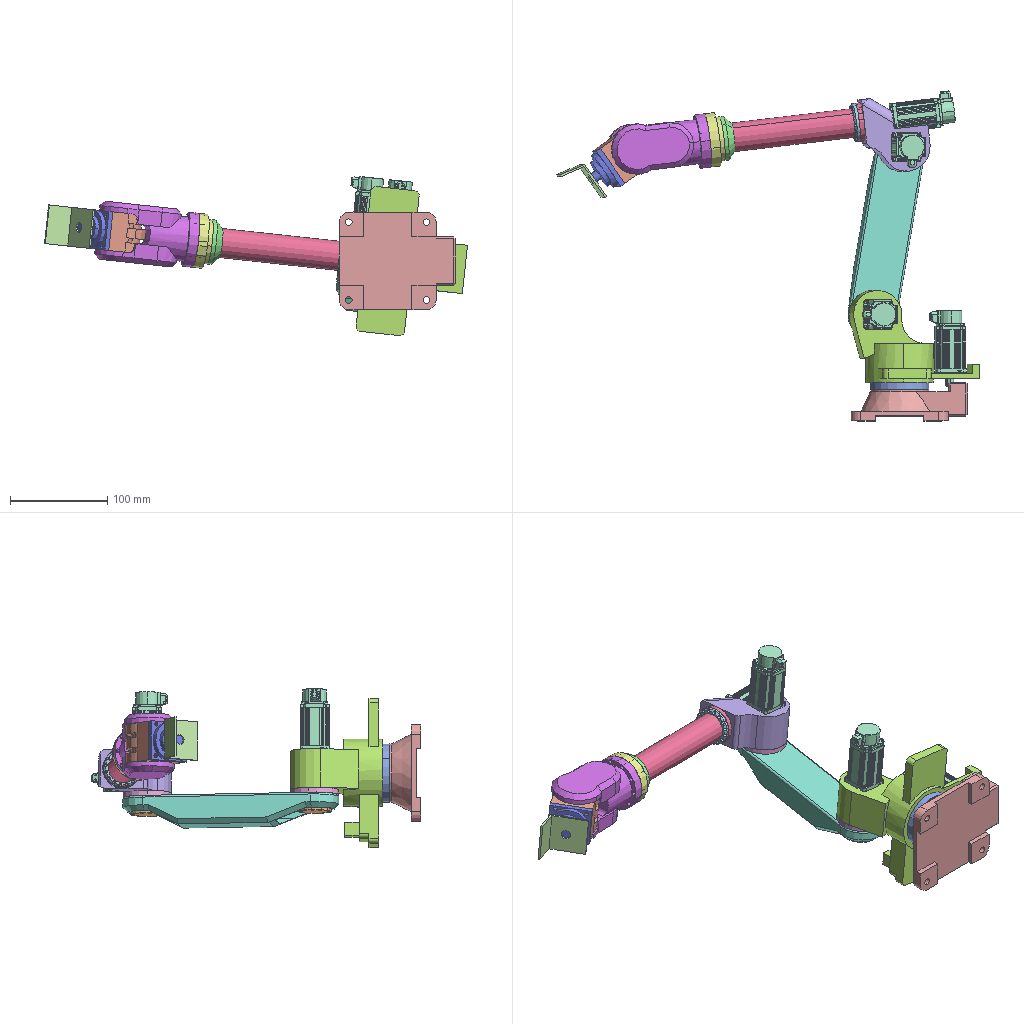Assembly | SolidWorks | 12 different items | 17 placed | box 436 x 340 x 164 mm
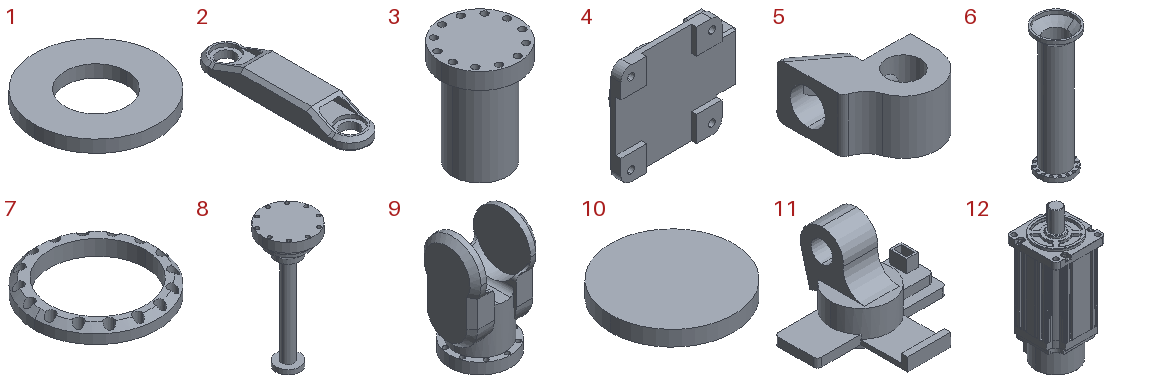Parts list (item | quantity | size | volume | features):
1 | x2 | 50 x 50 x 5 mm | 7363 mm3 | features Cut 1, Extrusion 1
2 | x1 | 50 x 225 x 30 mm | 173740 mm3 | features Cut 4, Fillet 2, Chamfer 1, Extrusion 1
3 | x2 | 35 x 35 x 47.5 mm | 26215 mm3 | features Cut 1, Extrusion 1, ICE 1
4 | x1 | 120 x 40 x 100 mm | 196028 mm3 | features ICE 3, Cut 2, Chamfer 1, Extrusion 1, Fillet 1, HoleWzd 1, Revolution 1
5 | x1 | 65 x 78.563 x 40 mm | 84441 mm3 | features Cut 5, Fillet 4, ICE 4, Extrusion 1
6 | x1 | 46 x 46 x 146.519 mm | 28748 mm3 | features Cut 3, Extrusion 1, ICE 1, Revolution 1
7 | x1 | 40 x 40 x 5 mm | 1718 mm3 | features Chamfer 1, Cut 1, Extrusion 1
8 | x1 | 56 x 56 x 136.215 mm | 62854 mm3 | features CirPattern 1, Cut 1, ICE 1, RevCut 1, Revolution 1
9 | x1 | 60 x 56 x 102.088 mm | 164993 mm3 | features Cut 3, ICE 2, Chamfer 1, CirPattern 1, Extrusion 1, Fillet 1, MirrorPattern 1
10 | x1 | 60 x 60 x 7.5 mm | 21206 mm3 | features Extrusion 1
11 | x1 | 150 x 130 x 95 mm | 315540 mm3 | features ICE 6, Fillet 4, Cut 2, Extrusion 1
12 | x4 | 30 x 36 x 78.5 mm | 46471 mm3 | features BaseBody 1, Scale 1
Mates (type | each side: item.copy, entity, surface, feature):
Concentric | 4.1 face cylinder Boss-Extrude2 | 10.1 face cylinder Boss-Extrude1
Coincident | 4.1 face plane Boss-Extrude2 | 10.1 face plane Boss-Extrude1
Concentric | 10.1 face cylinder Boss-Extrude1 | 11.1 face cylinder Boss-Extrude1
Coincident | 10.1 face plane Boss-Extrude1 | 11.1 face plane Boss-Extrude1
Concentric | 11.1 face cylinder Cut-Extrude1 | 1.1 face cylinder Boss-Extrude1
Coincident | 11.1 face plane Boss-Extrude6 | 1.1 face plane Boss-Extrude1
Coincident | 1.1 face plane Boss-Extrude1 | 2.1 face plane Boss-Extrude1
Concentric | 1.1 edge | 2.1 edge
Concentric | 11.1 face cylinder Cut-Extrude1 | 3.1 face cylinder Boss-Extrude2
Coincident | 2.1 face plane Cut-Extrude2 | 3.1 face plane Boss-Extrude1
Concentric | 2.1 face cylinder Cut-Extrude3 | 3.2 face cylinder Boss-Extrude2
Coincident | 2.1 face plane Cut-Extrude2 | 3.2 face plane Boss-Extrude1
Concentric | 3.2 face cylinder Boss-Extrude2 | 1.2 face cylinder Cut-Extrude1
Coincident | 2.1 face plane Boss-Extrude1 | 1.2 face plane Boss-Extrude1
Coincident | 3.2 face cylinder Boss-Extrude2 | 5.1 edge
Coincident | 1.2 face plane Boss-Extrude1 | 5.1 face plane Boss-Extrude1
Concentric | 6.1 face cylinder Boss-Extrude2 | 7.1 face cylinder Boss-Extrude1
Coincident | 6.1 face plane Boss-Extrude1 | 7.1 face plane Boss-Extrude1
Concentric | 6.1 face cylinder Cut-Extrude1 | 8.1 face cone Revolve1
InPlace | 8.1 face plane Revolve1 | assembly plane
Coincident | 11.1 face plane Boss-Extrude2 | 12.1 face plane Input1
Parallel | 11.1 face plane Boss-Extrude2 | 12.1 face plane Input1
Width | 11.1 face plane Boss-Extrude2 | 11.1 face plane Boss-Extrude2 | 12.1 face plane Input1 | 12.1 face plane Input1
DistanceDim | 12.1 face plane Input1 | 11.1 face plane Boss-Extrude3
Concentric | 11.1 face cylinder Cut-Extrude1 | 12.2 face cylinder Input1
Coincident | 11.1 face plane Boss-Extrude6 | 12.2 face plane Input1
Parallel | 11.1 face plane Boss-Extrude4 | 12.2 face plane Input1
Concentric | 5.1 face cylinder Cut-Extrude2 | 12.3 face cylinder Input1
Coincident | 5.1 face plane Boss-Extrude1 | 12.3 face plane Input1
Parallel | 12.2 face plane Input1 | 12.3 face plane Input1
Concentric | 6.1 face cylinder Cut-Extrude1 | 12.4 face cylinder Input1
Parallel | 5.1 face plane Boss-Extrude1 | 12.4 face plane Input1
Coincident | 5.1 face plane Boss-Extrude2 | 12.4 face plane Input1
Concentric | 5.1 face cylinder Cut-Extrude3 | 6.1 face cylinder Boss-Extrude2
Coincident | 5.1 face plane Boss-Extrude2 | 6.1 face plane Boss-Extrude1
Concentric | 8.1 face cone Revolve1 | 9.1 face cylinder Boss-Extrude1
Coincident | 8.1 face plane Revolve1 | 9.1 face plane Boss-Extrude1
Parallel | 2.1 face plane Boss-Extrude1 | 9.1 face plane Mirror1
InPlace | assembly plane | assembly plane
InPlace | assembly face | assembly plane
Coincident | 6.1 face plane Revolve1 | 8.1 face plane Revolve1